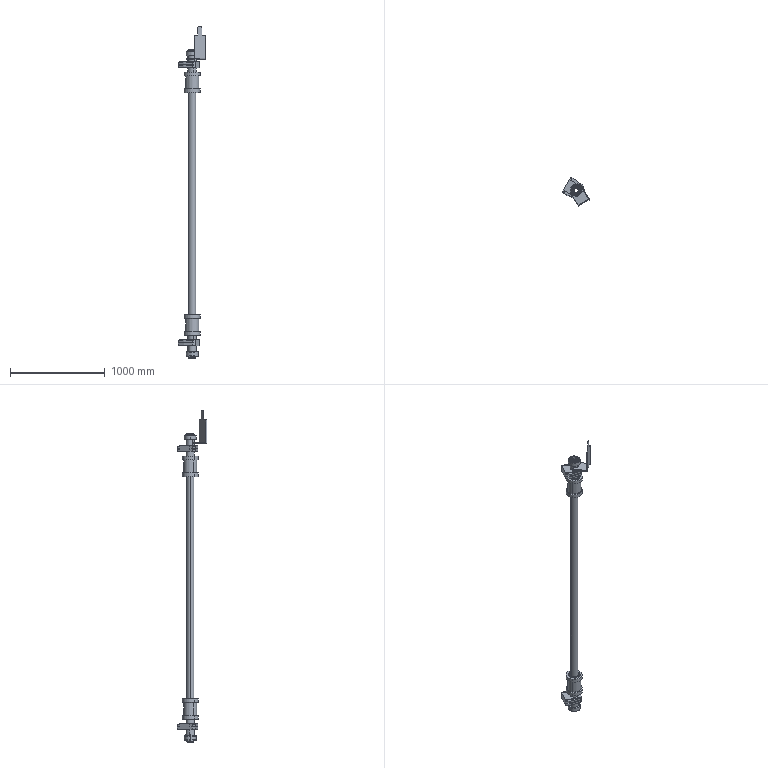Part | SolidWorks | features ReferencePattern 4, CompositeCurve 1, MirrorCompFeat 1 | 98 solids | 1320 faces | box 288.692 x 309.852 x 3501 mm | volume 17816483 mm3 | cylinder 468 | plane 378 | sphere 304 | torus 112 | cone 58 | commonest cylinder face diameters 94.75 x140 100.25 x140 70 x20 125 x20 8 x16 88.333 x16